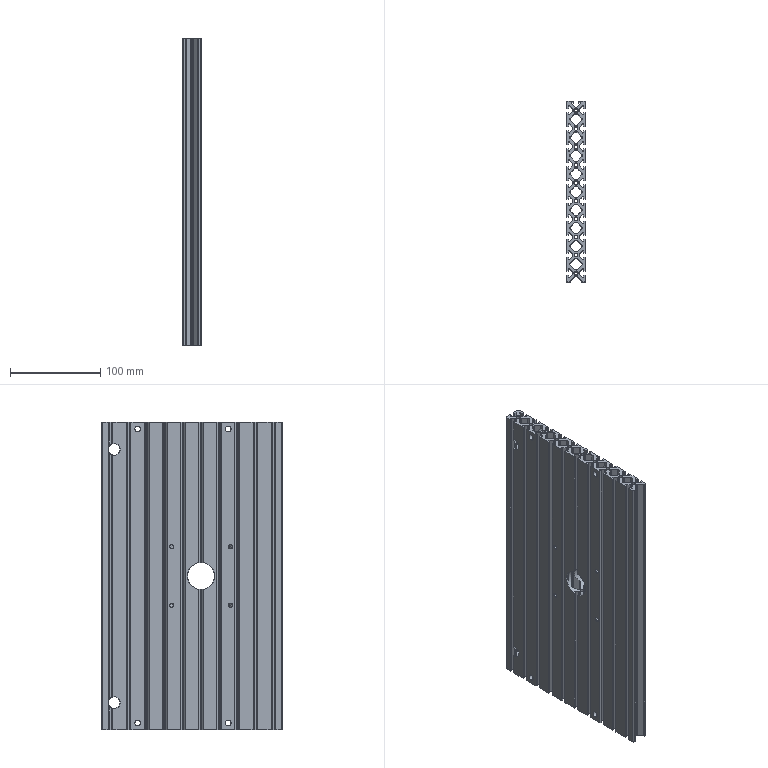Part | STEP file | 1 solid | 532 faces | box 20 x 200 x 340 mm | volume 654587 mm3 | plane 286 | cylinder 232 | cone 14 | commonest cylinder face diameters 2 x108 1 x50 4 x32 4.134 x14 4.2 x13 6.3 x8